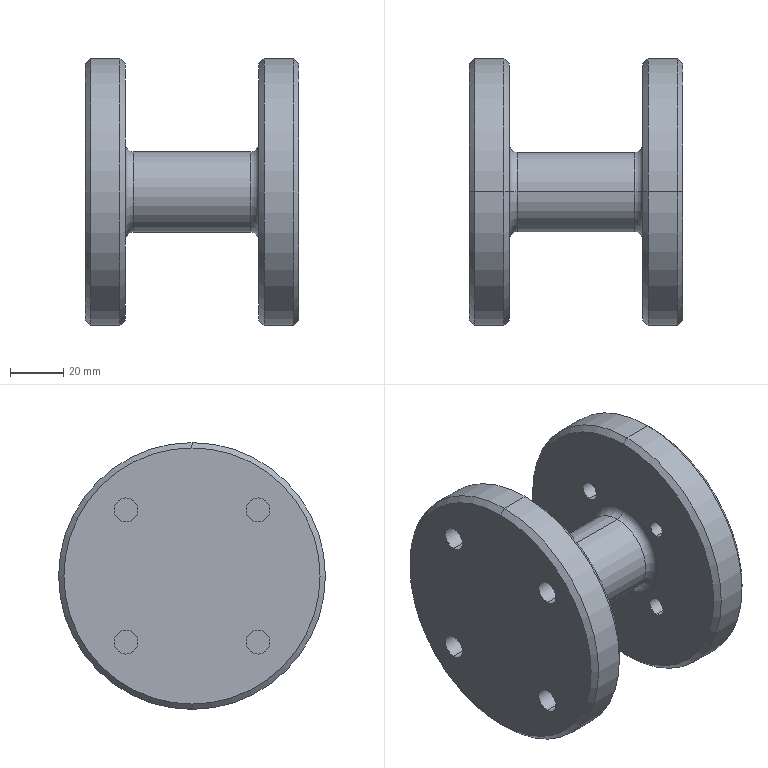Part | SolidWorks | features HoleWzd 3, ICE 2, Chamfer 1, CirPattern 1, Extrusion 1, Fillet 1 | 1 solid | 38 faces | box 80 x 100 x 100 mm | volume 263043 mm3 | cylinder 22 | cone 8 | torus 4 | plane 4 | commonest cylinder face diameters 9 x8 6 x4 7 x4 100 x4 30 x2
STEP:
#1=CARTESIAN_POINT('',(80.,0.,-48.));
#2=VERTEX_POINT('',#1);
#3=CARTESIAN_POINT('',(80.,0.,48.));
#4=VERTEX_POINT('',#3);
#5=CARTESIAN_POINT('',(80.,0.,0.));
#6=DIRECTION('',(1.,0.,0.));
#7=DIRECTION('',(0.,0.,-1.));
#8=AXIS2_PLACEMENT_3D('',#5,#6,#7);
#9=CIRCLE('',#8,48.);
#10=EDGE_CURVE('',#2,#4,#9,.T.);
#11=ORIENTED_EDGE('',*,*,#10,.F.);
#12=CARTESIAN_POINT('',(78.,0.,-50.));
#13=VERTEX_POINT('',#12);
#14=CARTESIAN_POINT('',(80.,0.,-48.));
#15=DIRECTION('',(-0.7071,0.,-0.7071));
#16=VECTOR('',#15,1000.);
#17=LINE('',#14,#16);
#18=EDGE_CURVE('',#2,#13,#17,.T.);
#19=ORIENTED_EDGE('',*,*,#18,.T.);
#20=CARTESIAN_POINT('',(78.,0.,50.));
#21=VERTEX_POINT('',#20);
#22=CARTESIAN_POINT('',(78.,0.,0.));
#23=DIRECTION('',(-1.,0.,0.));
#24=DIRECTION('',(0.,0.,-1.));
#25=AXIS2_PLACEMENT_3D('',#22,#23,#24);
#26=CIRCLE('',#25,50.);
#27=EDGE_CURVE('',#21,#13,#26,.T.);
#28=ORIENTED_EDGE('',*,*,#27,.F.);
#29=CARTESIAN_POINT('',(80.,0.,48.));
#30=DIRECTION('',(-0.7071,0.,0.7071));
#31=VECTOR('',#30,1000.);
#32=LINE('',#29,#31);
#33=EDGE_CURVE('',#4,#21,#32,.T.);
#34=ORIENTED_EDGE('',*,*,#33,.F.);
#35=EDGE_LOOP('',(#11,#19,#28,#34));
#36=FACE_OUTER_BOUND('',#35,.T.);
#37=CARTESIAN_POINT('',(80.,0.,0.));
#38=DIRECTION('',(-1.,0.,0.));
#39=DIRECTION('',(0.,0.,1.));
#40=AXIS2_PLACEMENT_3D('',#37,#38,#39);
#41=CONICAL_SURFACE('',#40,48.,0.7854);
#42=ADVANCED_FACE('',(#36),#41,.T.);
#43=CARTESIAN_POINT('',(65.,0.,48.));
#44=VERTEX_POINT('',#43);
#45=CARTESIAN_POINT('',(65.,0.,-48.));
#46=VERTEX_POINT('',#45);
#47=CARTESIAN_POINT('',(65.,0.,0.));
#48=DIRECTION('',(-1.,0.,0.));
#49=DIRECTION('',(0.,0.,-1.));
#50=AXIS2_PLACEMENT_3D('',#47,#48,#49);
#51=CIRCLE('',#50,48.);
#52=EDGE_CURVE('',#44,#46,#51,.T.);
#53=ORIENTED_EDGE('',*,*,#52,.F.);
#54=CARTESIAN_POINT('',(67.,0.,50.));
#55=VERTEX_POINT('',#54);
#56=CARTESIAN_POINT('',(67.,0.,50.));
#57=DIRECTION('',(0.7071,0.,0.7071));
#58=VECTOR('',#57,1000.);
#59=LINE('',#56,#58);
#60=EDGE_CURVE('',#44,#55,#59,.T.);
#61=ORIENTED_EDGE('',*,*,#60,.T.);
#62=CARTESIAN_POINT('',(67.,0.,-50.));
#63=VERTEX_POINT('',#62);
#64=CARTESIAN_POINT('',(67.,0.,0.));
#65=DIRECTION('',(1.,0.,0.));
#66=DIRECTION('',(0.,0.,-1.));
#67=AXIS2_PLACEMENT_3D('',#64,#65,#66);
#68=CIRCLE('',#67,50.);
#69=EDGE_CURVE('',#63,#55,#68,.T.);
#70=ORIENTED_EDGE('',*,*,#69,.F.);
#71=CARTESIAN_POINT('',(67.,0.,-50.));
#72=DIRECTION('',(0.7071,0.,-0.7071));
#73=VECTOR('',#72,1000.);
#74=LINE('',#71,#73);
#75=EDGE_CURVE('',#46,#63,#74,.T.);
#76=ORIENTED_EDGE('',*,*,#75,.F.);
#77=EDGE_LOOP('',(#53,#61,#70,#76));
#78=FACE_OUTER_BOUND('',#77,.T.);
#79=CARTESIAN_POINT('',(67.,0.,0.));
#80=DIRECTION('',(1.,0.,0.));
#81=DIRECTION('',(0.,0.,-1.));
#82=AXIS2_PLACEMENT_3D('',#79,#80,#81);
#83=CONICAL_SURFACE('',#82,50.,0.7854);
#84=ADVANCED_FACE('',(#78),#83,.T.);
#85=CARTESIAN_POINT('',(15.,0.,-48.));
#86=VERTEX_POINT('',#85);
#87=CARTESIAN_POINT('',(15.,0.,48.));
#88=VERTEX_POINT('',#87);
#89=CARTESIAN_POINT('',(15.,0.,0.));
#90=DIRECTION('',(1.,0.,0.));
#91=DIRECTION('',(0.,0.,-1.));
#92=AXIS2_PLACEMENT_3D('',#89,#90,#91);
#93=CIRCLE('',#92,48.);
#94=EDGE_CURVE('',#86,#88,#93,.T.);
#95=ORIENTED_EDGE('',*,*,#94,.F.);
#96=CARTESIAN_POINT('',(13.,0.,-50.));
#97=VERTEX_POINT('',#96);
#98=CARTESIAN_POINT('',(15.,0.,-48.));
#99=DIRECTION('',(-0.7071,0.,-0.7071));
#100=VECTOR('',#99,1000.);
#101=LINE('',#98,#100);
#102=EDGE_CURVE('',#86,#97,#101,.T.);
#103=ORIENTED_EDGE('',*,*,#102,.T.);
#104=CARTESIAN_POINT('',(13.,0.,50.));
#105=VERTEX_POINT('',#104);
#106=CARTESIAN_POINT('',(13.,0.,0.));
#107=DIRECTION('',(-1.,0.,0.));
#108=DIRECTION('',(0.,0.,-1.));
#109=AXIS2_PLACEMENT_3D('',#106,#107,#108);
#110=CIRCLE('',#109,50.);
#111=EDGE_CURVE('',#105,#97,#110,.T.);
#112=ORIENTED_EDGE('',*,*,#111,.F.);
#113=CARTESIAN_POINT('',(15.,0.,48.));
#114=DIRECTION('',(-0.7071,0.,0.7071));
#115=VECTOR('',#114,1000.);
#116=LINE('',#113,#115);
#117=EDGE_CURVE('',#88,#105,#116,.T.);
#118=ORIENTED_EDGE('',*,*,#117,.F.);
#119=EDGE_LOOP('',(#95,#103,#112,#118));
#120=FACE_OUTER_BOUND('',#119,.T.);
#121=CARTESIAN_POINT('',(15.,0.,0.));
#122=DIRECTION('',(-1.,0.,0.));
#123=DIRECTION('',(0.,0.,1.));
#124=AXIS2_PLACEMENT_3D('',#121,#122,#123);
#125=CONICAL_SURFACE('',#124,48.,0.7854);
#126=ADVANCED_FACE('',(#120),#125,.T.);
#127=CARTESIAN_POINT('',(0.,0.,48.));
#128=VERTEX_POINT('',#127);
#129=CARTESIAN_POINT('',(0.,0.,-48.));
#130=VERTEX_POINT('',#129);
#131=CARTESIAN_POINT('',(0.,0.,0.));
#132=DIRECTION('',(-1.,0.,0.));
#133=DIRECTION('',(0.,0.,-1.));
#134=AXIS2_PLACEMENT_3D('',#131,#132,#133);
#135=CIRCLE('',#134,48.);
#136=EDGE_CURVE('',#128,#130,#135,.T.);
#137=ORIENTED_EDGE('',*,*,#136,.F.);
#138=CARTESIAN_POINT('',(2.,0.,50.));
#139=VERTEX_POINT('',#138);
#140=CARTESIAN_POINT('',(2.,0.,50.));
#141=DIRECTION('',(0.7071,0.,0.7071));
#142=VECTOR('',#141,1000.);
#143=LINE('',#140,#142);
#144=EDGE_CURVE('',#128,#139,#143,.T.);
#145=ORIENTED_EDGE('',*,*,#144,.T.);
#146=CARTESIAN_POINT('',(2.,0.,-50.));
#147=VERTEX_POINT('',#146);
#148=CARTESIAN_POINT('',(2.,0.,0.));
#149=DIRECTION('',(1.,0.,0.));
#150=DIRECTION('',(0.,0.,-1.));
#151=AXIS2_PLACEMENT_3D('',#148,#149,#150);
#152=CIRCLE('',#151,50.);
#153=EDGE_CURVE('',#147,#139,#152,.T.);
#154=ORIENTED_EDGE('',*,*,#153,.F.);
#155=CARTESIAN_POINT('',(2.,0.,-50.));
#156=DIRECTION('',(0.7071,0.,-0.7071));
#157=VECTOR('',#156,1000.);
#158=LINE('',#155,#157);
#159=EDGE_CURVE('',#130,#147,#158,.T.);
#160=ORIENTED_EDGE('',*,*,#159,.F.);
#161=EDGE_LOOP('',(#137,#145,#154,#160));
#162=FACE_OUTER_BOUND('',#161,.T.);
#163=CARTESIAN_POINT('',(2.,0.,0.));
#164=DIRECTION('',(1.,0.,0.));
#165=DIRECTION('',(0.,0.,-1.));
#166=AXIS2_PLACEMENT_3D('',#163,#164,#165);
#167=CONICAL_SURFACE('',#166,50.,0.7854);
#168=ADVANCED_FACE('',(#162),#167,.T.);
#169=CARTESIAN_POINT('',(65.,0.,18.));
#170=VERTEX_POINT('',#169);
#171=CARTESIAN_POINT('',(65.,0.,-18.));
#172=VERTEX_POINT('',#171);
#173=CARTESIAN_POINT('',(65.,0.,0.));
#174=DIRECTION('',(1.,0.,0.));
#175=DIRECTION('',(0.,0.,-1.));
#176=AXIS2_PLACEMENT_3D('',#173,#174,#175);
#177=CIRCLE('',#176,18.);
#178=EDGE_CURVE('',#170,#172,#177,.T.);
#179=ORIENTED_EDGE('',*,*,#178,.F.);
#180=CARTESIAN_POINT('',(62.,0.,15.));
#181=VERTEX_POINT('',#180);
#182=CARTESIAN_POINT('',(62.,0.,18.));
#183=DIRECTION('',(0.,1.,0.));
#184=DIRECTION('',(0.,0.,1.));
#185=AXIS2_PLACEMENT_3D('',#182,#183,#184);
#186=CIRCLE('',#185,3.);
#187=EDGE_CURVE('',#170,#181,#186,.T.);
#188=ORIENTED_EDGE('',*,*,#187,.T.);
#189=CARTESIAN_POINT('',(62.,0.,-15.));
#190=VERTEX_POINT('',#189);
#191=CARTESIAN_POINT('',(62.,0.,0.));
#192=DIRECTION('',(-1.,0.,0.));
#193=DIRECTION('',(0.,0.,-1.));
#194=AXIS2_PLACEMENT_3D('',#191,#192,#193);
#195=CIRCLE('',#194,15.);
#196=EDGE_CURVE('',#190,#181,#195,.T.);
#197=ORIENTED_EDGE('',*,*,#196,.F.);
#198=CARTESIAN_POINT('',(62.,0.,-18.));
#199=DIRECTION('',(0.,-1.,0.));
#200=DIRECTION('',(0.,0.,-1.));
#201=AXIS2_PLACEMENT_3D('',#198,#199,#200);
#202=CIRCLE('',#201,3.);
#203=EDGE_CURVE('',#172,#190,#202,.T.);
#204=ORIENTED_EDGE('',*,*,#203,.F.);
#205=EDGE_LOOP('',(#179,#188,#197,#204));
#206=FACE_OUTER_BOUND('',#205,.T.);
#207=CARTESIAN_POINT('',(62.,0.,0.));
#208=DIRECTION('',(1.,0.,0.));
#209=DIRECTION('',(0.,0.,-1.));
#210=AXIS2_PLACEMENT_3D('',#207,#208,#209);
#211=TOROIDAL_SURFACE('',#210,18.,3.);
#212=ADVANCED_FACE('',(#206),#211,.F.);
#213=CARTESIAN_POINT('',(18.,0.,15.));
#214=VERTEX_POINT('',#213);
#215=CARTESIAN_POINT('',(18.,0.,-15.));
#216=VERTEX_POINT('',#215);
#217=CARTESIAN_POINT('',(18.,0.,0.));
#218=DIRECTION('',(1.,0.,0.));
#219=DIRECTION('',(0.,0.,-1.));
#220=AXIS2_PLACEMENT_3D('',#217,#218,#219);
#221=CIRCLE('',#220,15.);
#222=EDGE_CURVE('',#214,#216,#221,.T.);
#223=ORIENTED_EDGE('',*,*,#222,.F.);
#224=CARTESIAN_POINT('',(15.,0.,18.));
#225=VERTEX_POINT('',#224);
#226=CARTESIAN_POINT('',(18.,0.,18.));
#227=DIRECTION('',(0.,1.,0.));
#228=DIRECTION('',(0.,0.,1.));
#229=AXIS2_PLACEMENT_3D('',#226,#227,#228);
#230=CIRCLE('',#229,3.);
#231=EDGE_CURVE('',#214,#225,#230,.T.);
#232=ORIENTED_EDGE('',*,*,#231,.T.);
#233=CARTESIAN_POINT('',(15.,0.,-18.));
#234=VERTEX_POINT('',#233);
#235=CARTESIAN_POINT('',(15.,0.,0.));
#236=DIRECTION('',(-1.,0.,0.));
#237=DIRECTION('',(0.,0.,-1.));
#238=AXIS2_PLACEMENT_3D('',#235,#236,#237);
#239=CIRCLE('',#238,18.);
#240=EDGE_CURVE('',#234,#225,#239,.T.);
#241=ORIENTED_EDGE('',*,*,#240,.F.);
#242=CARTESIAN_POINT('',(18.,0.,-18.));
#243=DIRECTION('',(0.,-1.,0.));
#244=DIRECTION('',(0.,0.,-1.));
#245=AXIS2_PLACEMENT_3D('',#242,#243,#244);
#246=CIRCLE('',#245,3.);
#247=EDGE_CURVE('',#216,#234,#246,.T.);
#248=ORIENTED_EDGE('',*,*,#247,.F.);
#249=EDGE_LOOP('',(#223,#232,#241,#248));
#250=FACE_OUTER_BOUND('',#249,.T.);
#251=CARTESIAN_POINT('',(18.,0.,0.));
#252=DIRECTION('',(1.,0.,0.));
#253=DIRECTION('',(0.,0.,-1.));
#254=AXIS2_PLACEMENT_3D('',#251,#252,#253);
#255=TOROIDAL_SURFACE('',#254,18.,3.);
#256=ADVANCED_FACE('',(#250),#255,.F.);
#257=CARTESIAN_POINT('',(15.,24.749,29.249));
#258=VERTEX_POINT('',#257);
#259=CARTESIAN_POINT('',(15.,24.749,20.249));
#260=VERTEX_POINT('',#259);
#261=CARTESIAN_POINT('',(15.,24.749,24.749));
#262=DIRECTION('',(1.,0.,0.));
#263=DIRECTION('',(0.,0.,-1.));
#264=AXIS2_PLACEMENT_3D('',#261,#262,#263);
#265=CIRCLE('',#264,4.5);
#266=EDGE_CURVE('',#258,#260,#265,.T.);
#267=ORIENTED_EDGE('',*,*,#266,.T.);
#268=CARTESIAN_POINT('',(0.,24.749,20.249));
#269=VERTEX_POINT('',#268);
#270=CARTESIAN_POINT('',(0.,24.749,20.249));
#271=DIRECTION('',(-1.,0.,0.));
#272=VECTOR('',#271,1000.);
#273=LINE('',#270,#272);
#274=EDGE_CURVE('',#260,#269,#273,.T.);
#275=ORIENTED_EDGE('',*,*,#274,.T.);
#276=CARTESIAN_POINT('',(0.,24.749,29.249));
#277=VERTEX_POINT('',#276);
#278=CARTESIAN_POINT('',(0.,24.749,24.749));
#279=DIRECTION('',(-1.,0.,0.));
#280=DIRECTION('',(0.,0.,1.));
#281=AXIS2_PLACEMENT_3D('',#278,#279,#280);
#282=CIRCLE('',#281,4.5);
#283=EDGE_CURVE('',#269,#277,#282,.T.);
#284=ORIENTED_EDGE('',*,*,#283,.T.);
#285=CARTESIAN_POINT('',(0.,24.749,29.249));
#286=DIRECTION('',(-1.,0.,0.));
#287=VECTOR('',#286,1000.);
#288=LINE('',#285,#287);
#289=EDGE_CURVE('',#258,#277,#288,.T.);
#290=ORIENTED_EDGE('',*,*,#289,.F.);
#291=EDGE_LOOP('',(#267,#275,#284,#290));
#292=FACE_OUTER_BOUND('',#291,.T.);
#293=CARTESIAN_POINT('',(0.,24.749,24.749));
#294=DIRECTION('',(-1.,0.,0.));
#295=DIRECTION('',(0.,0.,1.));
#296=AXIS2_PLACEMENT_3D('',#293,#294,#295);
#297=CYLINDRICAL_SURFACE('',#296,4.5);
#298=ADVANCED_FACE('',(#292),#297,.F.);
#299=CARTESIAN_POINT('',(15.,-24.749,29.249));
#300=VERTEX_POINT('',#299);
#301=CARTESIAN_POINT('',(15.,-24.749,20.249));
#302=VERTEX_POINT('',#301);
#303=CARTESIAN_POINT('',(15.,-24.749,24.749));
#304=DIRECTION('',(1.,0.,0.));
#305=DIRECTION('',(0.,0.,-1.));
#306=AXIS2_PLACEMENT_3D('',#303,#304,#305);
#307=CIRCLE('',#306,4.5);
#308=EDGE_CURVE('',#300,#302,#307,.T.);
#309=ORIENTED_EDGE('',*,*,#308,.T.);
#310=CARTESIAN_POINT('',(0.,-24.749,20.249));
#311=VERTEX_POINT('',#310);
#312=CARTESIAN_POINT('',(0.,-24.749,20.249));
#313=DIRECTION('',(-1.,0.,0.));
#314=VECTOR('',#313,1000.);
#315=LINE('',#312,#314);
#316=EDGE_CURVE('',#302,#311,#315,.T.);
#317=ORIENTED_EDGE('',*,*,#316,.T.);
#318=CARTESIAN_POINT('',(0.,-24.749,29.249));
#319=VERTEX_POINT('',#318);
#320=CARTESIAN_POINT('',(0.,-24.749,24.749));
#321=DIRECTION('',(-1.,0.,0.));
#322=DIRECTION('',(0.,0.,1.));
#323=AXIS2_PLACEMENT_3D('',#320,#321,#322);
#324=CIRCLE('',#323,4.5);
#325=EDGE_CURVE('',#311,#319,#324,.T.);
#326=ORIENTED_EDGE('',*,*,#325,.T.);
#327=CARTESIAN_POINT('',(0.,-24.749,29.249));
#328=DIRECTION('',(-1.,0.,0.));
#329=VECTOR('',#328,1000.);
#330=LINE('',#327,#329);
#331=EDGE_CURVE('',#300,#319,#330,.T.);
#332=ORIENTED_EDGE('',*,*,#331,.F.);
#333=EDGE_LOOP('',(#309,#317,#326,#332));
#334=FACE_OUTER_BOUND('',#333,.T.);
#335=CARTESIAN_POINT('',(0.,-24.749,24.749));
#336=DIRECTION('',(-1.,0.,0.));
#337=DIRECTION('',(0.,0.,1.));
#338=AXIS2_PLACEMENT_3D('',#335,#336,#337);
#339=CYLINDRICAL_SURFACE('',#338,4.5);
#340=ADVANCED_FACE('',(#334),#339,.F.);
#341=CARTESIAN_POINT('',(15.,-24.749,-20.249));
#342=VERTEX_POINT('',#341);
#343=CARTESIAN_POINT('',(15.,-24.749,-29.249));
#344=VERTEX_POINT('',#343);
#345=CARTESIAN_POINT('',(15.,-24.749,-24.749));
#346=DIRECTION('',(1.,0.,0.));
#347=DIRECTION('',(0.,0.,-1.));
#348=AXIS2_PLACEMENT_3D('',#345,#346,#347);
#349=CIRCLE('',#348,4.5);
#350=EDGE_CURVE('',#342,#344,#349,.T.);
#351=ORIENTED_EDGE('',*,*,#350,.T.);
#352=CARTESIAN_POINT('',(0.,-24.749,-29.249));
#353=VERTEX_POINT('',#352);
#354=CARTESIAN_POINT('',(0.,-24.749,-29.249));
#355=DIRECTION('',(-1.,0.,0.));
#356=VECTOR('',#355,1000.);
#357=LINE('',#354,#356);
#358=EDGE_CURVE('',#344,#353,#357,.T.);
#359=ORIENTED_EDGE('',*,*,#358,.T.);
#360=CARTESIAN_POINT('',(0.,-24.749,-20.249));
#361=VERTEX_POINT('',#360);
#362=CARTESIAN_POINT('',(0.,-24.749,-24.749));
#363=DIRECTION('',(-1.,0.,0.));
#364=DIRECTION('',(0.,0.,1.));
#365=AXIS2_PLACEMENT_3D('',#362,#363,#364);
#366=CIRCLE('',#365,4.5);
#367=EDGE_CURVE('',#353,#361,#366,.T.);
#368=ORIENTED_EDGE('',*,*,#367,.T.);
#369=CARTESIAN_POINT('',(0.,-24.749,-20.249));
#370=DIRECTION('',(-1.,0.,0.));
#371=VECTOR('',#370,1000.);
#372=LINE('',#369,#371);
#373=EDGE_CURVE('',#342,#361,#372,.T.);
#374=ORIENTED_EDGE('',*,*,#373,.F.);
#375=EDGE_LOOP('',(#351,#359,#368,#374));
#376=FACE_OUTER_BOUND('',#375,.T.);
#377=CARTESIAN_POINT('',(0.,-24.749,-24.749));
#378=DIRECTION('',(-1.,0.,0.));
#379=DIRECTION('',(0.,0.,1.));
#380=AXIS2_PLACEMENT_3D('',#377,#378,#379);
#381=CYLINDRICAL_SURFACE('',#380,4.5);
#382=ADVANCED_FACE('',(#376),#381,.F.);
#383=CARTESIAN_POINT('',(15.,24.749,-20.249));
#384=VERTEX_POINT('',#383);
#385=CARTESIAN_POINT('',(15.,24.749,-29.249));
#386=VERTEX_POINT('',#385);
#387=CARTESIAN_POINT('',(15.,24.749,-24.749));
#388=DIRECTION('',(1.,0.,0.));
#389=DIRECTION('',(0.,0.,-1.));
#390=AXIS2_PLACEMENT_3D('',#387,#388,#389);
#391=CIRCLE('',#390,4.5);
#392=EDGE_CURVE('',#384,#386,#391,.T.);
#393=ORIENTED_EDGE('',*,*,#392,.T.);
#394=CARTESIAN_POINT('',(0.,24.749,-29.249));
#395=VERTEX_POINT('',#394);
#396=CARTESIAN_POINT('',(0.,24.749,-29.249));
#397=DIRECTION('',(-1.,0.,0.));
#398=VECTOR('',#397,1000.);
#399=LINE('',#396,#398);
#400=EDGE_CURVE('',#386,#395,#399,.T.);
#401=ORIENTED_EDGE('',*,*,#400,.T.);
#402=CARTESIAN_POINT('',(0.,24.749,-20.249));
#403=VERTEX_POINT('',#402);
#404=CARTESIAN_POINT('',(0.,24.749,-24.749));
#405=DIRECTION('',(-1.,0.,0.));
#406=DIRECTION('',(0.,0.,1.));
#407=AXIS2_PLACEMENT_3D('',#404,#405,#406);
#408=CIRCLE('',#407,4.5);
#409=EDGE_CURVE('',#395,#403,#408,.T.);
#410=ORIENTED_EDGE('',*,*,#409,.T.);
#411=CARTESIAN_POINT('',(0.,24.749,-20.249));
#412=DIRECTION('',(-1.,0.,0.));
#413=VECTOR('',#412,1000.);
#414=LINE('',#411,#413);
#415=EDGE_CURVE('',#384,#403,#414,.T.);
#416=ORIENTED_EDGE('',*,*,#415,.F.);
#417=EDGE_LOOP('',(#393,#401,#410,#416));
#418=FACE_OUTER_BOUND('',#417,.T.);
#419=CARTESIAN_POINT('',(0.,24.749,-24.749));
#420=DIRECTION('',(-1.,0.,0.));
#421=DIRECTION('',(0.,0.,1.));
#422=AXIS2_PLACEMENT_3D('',#419,#420,#421);
#423=CYLINDRICAL_SURFACE('',#422,4.5);
#424=ADVANCED_FACE('',(#418),#423,.F.);
#425=CARTESIAN_POINT('',(65.,-17.699,20.699));
#426=VERTEX_POINT('',#425);
#427=CARTESIAN_POINT('',(65.,-17.699,14.699));
#428=VERTEX_POINT('',#427);
#429=CARTESIAN_POINT('',(65.,-17.699,17.699));
#430=DIRECTION('',(1.,0.,0.));
#431=DIRECTION('',(0.,0.,-1.));
#432=AXIS2_PLACEMENT_3D('',#429,#430,#431);
#433=CIRCLE('',#432,3.);
#434=EDGE_CURVE('',#426,#428,#433,.T.);
#435=ORIENTED_EDGE('',*,*,#434,.F.);
#436=CARTESIAN_POINT('',(80.,-17.699,20.699));
#437=VERTEX_POINT('',#436);
#438=CARTESIAN_POINT('',(80.,-17.699,20.699));
#439=DIRECTION('',(1.,0.,0.));
#440=VECTOR('',#439,1000.);
#441=LINE('',#438,#440);
#442=EDGE_CURVE('',#426,#437,#441,.T.);
#443=ORIENTED_EDGE('',*,*,#442,.T.);
#444=CARTESIAN_POINT('',(80.,-17.699,14.699));
#445=VERTEX_POINT('',#444);
#446=CARTESIAN_POINT('',(80.,-17.699,17.699));
#447=DIRECTION('',(1.,0.,0.));
#448=DIRECTION('',(0.,0.,-1.));
#449=AXIS2_PLACEMENT_3D('',#446,#447,#448);
#450=CIRCLE('',#449,3.);
#451=EDGE_CURVE('',#437,#445,#450,.T.);
#452=ORIENTED_EDGE('',*,*,#451,.T.);
#453=CARTESIAN_POINT('',(80.,-17.699,14.699));
#454=DIRECTION('',(1.,0.,0.));
#455=VECTOR('',#454,1000.);
#456=LINE('',#453,#455);
#457=EDGE_CURVE('',#428,#445,#456,.T.);
#458=ORIENTED_EDGE('',*,*,#457,.F.);
#459=EDGE_LOOP('',(#435,#443,#452,#458));
#460=FACE_OUTER_BOUND('',#459,.T.);
#461=CARTESIAN_POINT('',(80.,-17.699,17.699));
#462=DIRECTION('',(1.,0.,0.));
#463=DIRECTION('',(0.,0.,-1.));
#464=AXIS2_PLACEMENT_3D('',#461,#462,#463);
#465=CYLINDRICAL_SURFACE('',#464,3.);
#466=ADVANCED_FACE('',(#460),#465,.F.);
#467=CARTESIAN_POINT('',(65.,17.699,-14.699));
#468=VERTEX_POINT('',#467);
#469=CARTESIAN_POINT('',(65.,17.699,-20.699));
#470=VERTEX_POINT('',#469);
#471=CARTESIAN_POINT('',(65.,17.699,-17.699));
#472=DIRECTION('',(1.,0.,0.));
#473=DIRECTION('',(0.,0.,-1.));
#474=AXIS2_PLACEMENT_3D('',#471,#472,#473);
#475=CIRCLE('',#474,3.);
#476=EDGE_CURVE('',#468,#470,#475,.T.);
#477=ORIENTED_EDGE('',*,*,#476,.F.);
#478=CARTESIAN_POINT('',(80.,17.699,-14.699));
#479=VERTEX_POINT('',#478);
#480=CARTESIAN_POINT('',(80.,17.699,-14.699));
#481=DIRECTION('',(1.,0.,0.));
#482=VECTOR('',#481,1000.);
#483=LINE('',#480,#482);
#484=EDGE_CURVE('',#468,#479,#483,.T.);
#485=ORIENTED_EDGE('',*,*,#484,.T.);
#486=CARTESIAN_POINT('',(80.,17.699,-20.699));
#487=VERTEX_POINT('',#486);
#488=CARTESIAN_POINT('',(80.,17.699,-17.699));
#489=DIRECTION('',(1.,0.,0.));
#490=DIRECTION('',(0.,0.,-1.));
#491=AXIS2_PLACEMENT_3D('',#488,#489,#490);
#492=CIRCLE('',#491,3.);
#493=EDGE_CURVE('',#479,#487,#492,.T.);
#494=ORIENTED_EDGE('',*,*,#493,.T.);
#495=CARTESIAN_POINT('',(80.,17.699,-20.699));
#496=DIRECTION('',(1.,0.,0.));
#497=VECTOR('',#496,1000.);
#498=LINE('',#495,#497);
#499=EDGE_CURVE('',#470,#487,#498,.T.);
#500=ORIENTED_EDGE('',*,*,#499,.F.);
#501=EDGE_LOOP('',(#477,#485,#494,#500));
#502=FACE_OUTER_BOUND('',#501,.T.);
#503=CARTESIAN_POINT('',(80.,17.699,-17.699));
#504=DIRECTION('',(1.,0.,0.));
#505=DIRECTION('',(0.,0.,-1.));
#506=AXIS2_PLACEMENT_3D('',#503,#504,#505);
#507=CYLINDRICAL_SURFACE('',#506,3.);
#508=ADVANCED_FACE('',(#502),#507,.F.);
#509=CARTESIAN_POINT('',(65.,17.699,21.199));
#510=VERTEX_POINT('',#509);
#511=CARTESIAN_POINT('',(65.,17.699,14.199));
#512=VERTEX_POINT('',#511);
#513=CARTESIAN_POINT('',(65.,17.699,17.699));
#514=DIRECTION('',(1.,0.,0.));
#515=DIRECTION('',(0.,0.,-1.));
#516=AXIS2_PLACEMENT_3D('',#513,#514,#515);
#517=CIRCLE('',#516,3.5);
#518=EDGE_CURVE('',#510,#512,#517,.T.);
#519=ORIENTED_EDGE('',*,*,#518,.F.);
#520=CARTESIAN_POINT('',(80.,17.699,21.199));
#521=VERTEX_POINT('',#520);
#522=CARTESIAN_POINT('',(80.,17.699,21.199));
#523=DIRECTION('',(1.,0.,0.));
#524=VECTOR('',#523,1000.);
#525=LINE('',#522,#524);
#526=EDGE_CURVE('',#510,#521,#525,.T.);
#527=ORIENTED_EDGE('',*,*,#526,.T.);
#528=CARTESIAN_POINT('',(80.,17.699,14.199));
#529=VERTEX_POINT('',#528);
#530=CARTESIAN_POINT('',(80.,17.699,17.699));
#531=DIRECTION('',(1.,0.,0.));
#532=DIRECTION('',(0.,0.,-1.));
#533=AXIS2_PLACEMENT_3D('',#530,#531,#532);
#534=CIRCLE('',#533,3.5);
#535=EDGE_CURVE('',#521,#529,#534,.T.);
#536=ORIENTED_EDGE('',*,*,#535,.T.);
#537=CARTESIAN_POINT('',(80.,17.699,14.199));
#538=DIRECTION('',(1.,0.,0.));
#539=VECTOR('',#538,1000.);
#540=LINE('',#537,#539);
#541=EDGE_CURVE('',#512,#529,#540,.T.);
#542=ORIENTED_EDGE('',*,*,#541,.F.);
#543=EDGE_LOOP('',(#519,#527,#536,#542));
#544=FACE_OUTER_BOUND('',#543,.T.);
#545=CARTESIAN_POINT('',(80.,17.699,17.699));
#546=DIRECTION('',(1.,0.,0.));
#547=DIRECTION('',(0.,0.,-1.));
#548=AXIS2_PLACEMENT_3D('',#545,#546,#547);
#549=CYLINDRICAL_SURFACE('',#548,3.5);
#550=ADVANCED_FACE('',(#544),#549,.F.);
#551=CARTESIAN_POINT('',(65.,-17.699,-14.199));
#552=VERTEX_POINT('',#551);
#553=CARTESIAN_POINT('',(65.,-17.699,-21.199));
#554=VERTEX_POINT('',#553);
#555=CARTESIAN_POINT('',(65.,-17.699,-17.699));
#556=DIRECTION('',(1.,0.,0.));
#557=DIRECTION('',(0.,0.,-1.));
#558=AXIS2_PLACEMENT_3D('',#555,#556,#557);
#559=CIRCLE('',#558,3.5);
#560=EDGE_CURVE('',#552,#554,#559,.T.);
#561=ORIENTED_EDGE('',*,*,#560,.F.);
#562=CARTESIAN_POINT('',(80.,-17.699,-14.199));
#563=VERTEX_POINT('',#562);
#564=CARTESIAN_POINT('',(80.,-17.699,-14.199));
#565=DIRECTION('',(1.,0.,0.));
#566=VECTOR('',#565,1000.);
#567=LINE('',#564,#566);
#568=EDGE_CURVE('',#552,#563,#567,.T.);
#569=ORIENTED_EDGE('',*,*,#568,.T.);
#570=CARTESIAN_POINT('',(80.,-17.699,-21.199));
#571=VERTEX_POINT('',#570);
#572=CARTESIAN_POINT('',(80.,-17.699,-17.699));
#573=DIRECTION('',(1.,0.,0.));
#574=DIRECTION('',(0.,0.,-1.));
#575=AXIS2_PLACEMENT_3D('',#572,#573,#574);
#576=CIRCLE('',#575,3.5);
#577=EDGE_CURVE('',#563,#571,#576,.T.);
#578=ORIENTED_EDGE('',*,*,#577,.T.);
#579=CARTESIAN_POINT('',(80.,-17.699,-21.199));
#580=DIRECTION('',(1.,0.,0.));
#581=VECTOR('',#580,1000.);
#582=LINE('',#579,#581);
#583=EDGE_CURVE('',#554,#571,#582,.T.);
#584=ORIENTED_EDGE('',*,*,#583,.F.);
#585=EDGE_LOOP('',(#561,#569,#578,#584));
#586=FACE_OUTER_BOUND('',#585,.T.);
#587=CARTESIAN_POINT('',(80.,-17.699,-17.699));
#588=DIRECTION('',(1.,0.,0.));
#589=DIRECTION('',(0.,0.,-1.));
#590=AXIS2_PLACEMENT_3D('',#587,#588,#589);
#591=CYLINDRICAL_SURFACE('',#590,3.5);
#592=ADVANCED_FACE('',(#586),#591,.F.);
#593=ORIENTED_EDGE('',*,*,#27,.T.);
#594=CARTESIAN_POINT('',(80.,0.,-50.));
#595=DIRECTION('',(-1.,0.,0.));
#596=VECTOR('',#595,1000.);
#597=LINE('',#594,#596);
#598=EDGE_CURVE('',#13,#63,#597,.T.);
#599=ORIENTED_EDGE('',*,*,#598,.T.);
#600=ORIENTED_EDGE('',*,*,#69,.T.);
#601=CARTESIAN_POINT('',(80.,0.,50.));
#602=DIRECTION('',(-1.,0.,0.));
#603=VECTOR('',#602,1000.);
#604=LINE('',#601,#603);
#605=EDGE_CURVE('',#21,#55,#604,.T.);
#606=ORIENTED_EDGE('',*,*,#605,.F.);
#607=EDGE_LOOP('',(#593,#599,#600,#606));
#608=FACE_OUTER_BOUND('',#607,.T.);
#609=CARTESIAN_POINT('',(80.,0.,0.));
#610=DIRECTION('',(-1.,0.,0.));
#611=DIRECTION('',(0.,0.,1.));
#612=AXIS2_PLACEMENT_3D('',#609,#610,#611);
#613=CYLINDRICAL_SURFACE('',#612,50.);
#614=ADVANCED_FACE('',(#608),#613,.T.);
#615=CARTESIAN_POINT('',(62.,0.,0.));
#616=DIRECTION('',(-1.,0.,0.));
#617=DIRECTION('',(0.,0.,-1.));
#618=AXIS2_PLACEMENT_3D('',#615,#616,#617);
#619=CIRCLE('',#618,15.);
#620=EDGE_CURVE('',#181,#190,#619,.T.);
#621=ORIENTED_EDGE('',*,*,#620,.T.);
#622=CARTESIAN_POINT('',(65.,0.,-15.));
#623=DIRECTION('',(-1.,0.,0.));
#624=VECTOR('',#623,1000.);
#625=LINE('',#622,#624);
#626=EDGE_CURVE('',#190,#216,#625,.T.);
#627=ORIENTED_EDGE('',*,*,#626,.T.);
#628=CARTESIAN_POINT('',(18.,0.,0.));
#629=DIRECTION('',(1.,0.,0.));
#630=DIRECTION('',(0.,0.,-1.));
#631=AXIS2_PLACEMENT_3D('',#628,#629,#630);
#632=CIRCLE('',#631,15.);
#633=EDGE_CURVE('',#216,#214,#632,.T.);
#634=ORIENTED_EDGE('',*,*,#633,.T.);
#635=CARTESIAN_POINT('',(65.,0.,15.));
#636=DIRECTION('',(-1.,0.,0.));
#637=VECTOR('',#636,1000.);
#638=LINE('',#635,#637);
#639=EDGE_CURVE('',#181,#214,#638,.T.);
#640=ORIENTED_EDGE('',*,*,#639,.F.);
#641=EDGE_LOOP('',(#621,#627,#634,#640));
#642=FACE_OUTER_BOUND('',#641,.T.);
#643=CARTESIAN_POINT('',(65.,0.,0.));
#644=DIRECTION('',(-1.,0.,0.));
#645=DIRECTION('',(0.,0.,1.));
#646=AXIS2_PLACEMENT_3D('',#643,#644,#645);
#647=CYLINDRICAL_SURFACE('',#646,15.);
#648=ADVANCED_FACE('',(#642),#647,.T.);
#649=ORIENTED_EDGE('',*,*,#111,.T.);
#650=CARTESIAN_POINT('',(15.,0.,-50.));
#651=DIRECTION('',(-1.,0.,0.));
#652=VECTOR('',#651,1000.);
#653=LINE('',#650,#652);
#654=EDGE_CURVE('',#97,#147,#653,.T.);
#655=ORIENTED_EDGE('',*,*,#654,.T.);
#656=ORIENTED_EDGE('',*,*,#153,.T.);
#657=CARTESIAN_POINT('',(15.,0.,50.));
#658=DIRECTION('',(-1.,0.,0.));
#659=VECTOR('',#658,1000.);
#660=LINE('',#657,#659);
#661=EDGE_CURVE('',#105,#139,#660,.T.);
#662=ORIENTED_EDGE('',*,*,#661,.F.);
#663=EDGE_LOOP('',(#649,#655,#656,#662));
#664=FACE_OUTER_BOUND('',#663,.T.);
#665=CARTESIAN_POINT('',(15.,0.,0.));
#666=DIRECTION('',(-1.,0.,0.));
#667=DIRECTION('',(0.,0.,1.));
#668=AXIS2_PLACEMENT_3D('',#665,#666,#667);
#669=CYLINDRICAL_SURFACE('',#668,50.);
#670=ADVANCED_FACE('',(#664),#669,.T.);
#671=ORIENTED_EDGE('',*,*,#654,.F.);
#672=CARTESIAN_POINT('',(13.,0.,0.));
#673=DIRECTION('',(-1.,0.,0.));
#674=DIRECTION('',(0.,0.,-1.));
#675=AXIS2_PLACEMENT_3D('',#672,#673,#674);
#676=CIRCLE('',#675,50.);
#677=EDGE_CURVE('',#97,#105,#676,.T.);
#678=ORIENTED_EDGE('',*,*,#677,.T.);
#679=ORIENTED_EDGE('',*,*,#661,.T.);
#680=CARTESIAN_POINT('',(2.,0.,0.));
#681=DIRECTION('',(1.,0.,0.));
#682=DIRECTION('',(0.,0.,-1.));
#683=AXIS2_PLACEMENT_3D('',#680,#681,#682);
#684=CIRCLE('',#683,50.);
#685=EDGE_CURVE('',#139,#147,#684,.T.);
#686=ORIENTED_EDGE('',*,*,#685,.T.);
#687=EDGE_LOOP('',(#671,#678,#679,#686));
#688=FACE_OUTER_BOUND('',#687,.T.);
#689=CARTESIAN_POINT('',(15.,0.,0.));
#690=DIRECTION('',(-1.,0.,0.));
#691=DIRECTION('',(0.,0.,1.));
#692=AXIS2_PLACEMENT_3D('',#689,#690,#691);
#693=CYLINDRICAL_SURFACE('',#692,50.);
#694=ADVANCED_FACE('',(#688),#693,.T.);
#695=CARTESIAN_POINT('',(15.,0.,0.));
#696=DIRECTION('',(1.,0.,0.));
#697=DIRECTION('',(0.,0.,-1.));
#698=AXIS2_PLACEMENT_3D('',#695,#696,#697);
#699=CIRCLE('',#698,48.);
#700=EDGE_CURVE('',#88,#86,#699,.T.);
#701=ORIENTED_EDGE('',*,*,#700,.T.);
#702=ORIENTED_EDGE('',*,*,#94,.T.);
#703=EDGE_LOOP('',(#701,#702));
#704=FACE_OUTER_BOUND('',#703,.T.);
#705=ORIENTED_EDGE('',*,*,#240,.T.);
#706=CARTESIAN_POINT('',(15.,0.,0.));
#707=DIRECTION('',(-1.,0.,0.));
#708=DIRECTION('',(0.,0.,-1.));
#709=AXIS2_PLACEMENT_3D('',#706,#707,#708);
#710=CIRCLE('',#709,18.);
#711=EDGE_CURVE('',#225,#234,#710,.T.);
#712=ORIENTED_EDGE('',*,*,#711,.T.);
#713=EDGE_LOOP('',(#705,#712));
#714=FACE_BOUND('',#713,.T.);
#715=ORIENTED_EDGE('',*,*,#266,.F.);
#716=CARTESIAN_POINT('',(15.,24.749,24.749));
#717=DIRECTION('',(1.,0.,0.));
#718=DIRECTION('',(0.,0.,-1.));
#719=AXIS2_PLACEMENT_3D('',#716,#717,#718);
#720=CIRCLE('',#719,4.5);
#721=EDGE_CURVE('',#260,#258,#720,.T.);
#722=ORIENTED_EDGE('',*,*,#721,.F.);
#723=EDGE_LOOP('',(#715,#722));
#724=FACE_BOUND('',#723,.T.);
#725=ORIENTED_EDGE('',*,*,#308,.F.);
#726=CARTESIAN_POINT('',(15.,-24.749,24.749));
#727=DIRECTION('',(1.,0.,0.));
#728=DIRECTION('',(0.,0.,-1.));
#729=AXIS2_PLACEMENT_3D('',#726,#727,#728);
#730=CIRCLE('',#729,4.5);
#731=EDGE_CURVE('',#302,#300,#730,.T.);
#732=ORIENTED_EDGE('',*,*,#731,.F.);
#733=EDGE_LOOP('',(#725,#732));
#734=FACE_BOUND('',#733,.T.);
#735=ORIENTED_EDGE('',*,*,#350,.F.);
#736=CARTESIAN_POINT('',(15.,-24.749,-24.749));
#737=DIRECTION('',(1.,0.,0.));
#738=DIRECTION('',(0.,0.,-1.));
#739=AXIS2_PLACEMENT_3D('',#736,#737,#738);
#740=CIRCLE('',#739,4.5);
#741=EDGE_CURVE('',#344,#342,#740,.T.);
#742=ORIENTED_EDGE('',*,*,#741,.F.);
#743=EDGE_LOOP('',(#735,#742));
#744=FACE_BOUND('',#743,.T.);
#745=ORIENTED_EDGE('',*,*,#392,.F.);
#746=CARTESIAN_POINT('',(15.,24.749,-24.749));
#747=DIRECTION('',(1.,0.,0.));
#748=DIRECTION('',(0.,0.,-1.));
#749=AXIS2_PLACEMENT_3D('',#746,#747,#748);
#750=CIRCLE('',#749,4.5);
#751=EDGE_CURVE('',#386,#384,#750,.T.);
#752=ORIENTED_EDGE('',*,*,#751,.F.);
#753=EDGE_LOOP('',(#745,#752));
#754=FACE_BOUND('',#753,.T.);
#755=CARTESIAN_POINT('',(15.,0.,0.));
#756=DIRECTION('',(1.,0.,0.));
#757=DIRECTION('',(0.,0.,-1.));
#758=AXIS2_PLACEMENT_3D('',#755,#756,#757);
#759=PLANE('',#758);
#760=ADVANCED_FACE('',(#704,#714,#724,#734,#744,#754),#759,.T.);
#761=CARTESIAN_POINT('',(0.,0.,0.));
#762=DIRECTION('',(-1.,0.,0.));
#763=DIRECTION('',(0.,0.,-1.));
#764=AXIS2_PLACEMENT_3D('',#761,#762,#763);
#765=CIRCLE('',#764,48.);
#766=EDGE_CURVE('',#130,#128,#765,.T.);
#767=ORIENTED_EDGE('',*,*,#766,.T.);
#768=ORIENTED_EDGE('',*,*,#136,.T.);
#769=EDGE_LOOP('',(#767,#768));
#770=FACE_OUTER_BOUND('',#769,.T.);
#771=CARTESIAN_POINT('',(0.,24.749,24.749));
#772=DIRECTION('',(-1.,0.,0.));
#773=DIRECTION('',(0.,0.,1.));
#774=AXIS2_PLACEMENT_3D('',#771,#772,#773);
#775=CIRCLE('',#774,4.5);
#776=EDGE_CURVE('',#277,#269,#775,.T.);
#777=ORIENTED_EDGE('',*,*,#776,.F.);
#778=ORIENTED_EDGE('',*,*,#283,.F.);
#779=EDGE_LOOP('',(#777,#778));
#780=FACE_BOUND('',#779,.T.);
#781=CARTESIAN_POINT('',(0.,-24.749,24.749));
#782=DIRECTION('',(-1.,0.,0.));
#783=DIRECTION('',(0.,0.,1.));
#784=AXIS2_PLACEMENT_3D('',#781,#782,#783);
#785=CIRCLE('',#784,4.5);
#786=EDGE_CURVE('',#319,#311,#785,.T.);
#787=ORIENTED_EDGE('',*,*,#786,.F.);
#788=ORIENTED_EDGE('',*,*,#325,.F.);
#789=EDGE_LOOP('',(#787,#788));
#790=FACE_BOUND('',#789,.T.);
#791=CARTESIAN_POINT('',(0.,-24.749,-24.749));
#792=DIRECTION('',(-1.,0.,0.));
#793=DIRECTION('',(0.,0.,1.));
#794=AXIS2_PLACEMENT_3D('',#791,#792,#793);
#795=CIRCLE('',#794,4.5);
#796=EDGE_CURVE('',#361,#353,#795,.T.);
#797=ORIENTED_EDGE('',*,*,#796,.F.);
#798=ORIENTED_EDGE('',*,*,#367,.F.);
#799=EDGE_LOOP('',(#797,#798));
#800=FACE_BOUND('',#799,.T.);
#801=CARTESIAN_POINT('',(0.,24.749,-24.749));
#802=DIRECTION('',(-1.,0.,0.));
#803=DIRECTION('',(0.,0.,1.));
#804=AXIS2_PLACEMENT_3D('',#801,#802,#803);
#805=CIRCLE('',#804,4.5);
#806=EDGE_CURVE('',#403,#395,#805,.T.);
#807=ORIENTED_EDGE('',*,*,#806,.F.);
#808=ORIENTED_EDGE('',*,*,#409,.F.);
#809=EDGE_LOOP('',(#807,#808));
#810=FACE_BOUND('',#809,.T.);
#811=CARTESIAN_POINT('',(0.,0.,0.));
#812=DIRECTION('',(1.,0.,0.));
#813=DIRECTION('',(0.,0.,-1.));
#814=AXIS2_PLACEMENT_3D('',#811,#812,#813);
#815=PLANE('',#814);
#816=ADVANCED_FACE('',(#770,#780,#790,#800,#810),#815,.F.);
#817=ORIENTED_EDGE('',*,*,#626,.F.);
#818=ORIENTED_EDGE('',*,*,#196,.T.);
#819=ORIENTED_EDGE('',*,*,#639,.T.);
#820=ORIENTED_EDGE('',*,*,#222,.T.);
#821=EDGE_LOOP('',(#817,#818,#819,#820));
#822=FACE_OUTER_BOUND('',#821,.T.);
#823=CARTESIAN_POINT('',(65.,0.,0.));
#824=DIRECTION('',(-1.,0.,0.));
#825=DIRECTION('',(0.,0.,1.));
#826=AXIS2_PLACEMENT_3D('',#823,#824,#825);
#827=CYLINDRICAL_SURFACE('',#826,15.);
#828=ADVANCED_FACE('',(#822),#827,.T.);
#829=ORIENTED_EDGE('',*,*,#598,.F.);
#830=CARTESIAN_POINT('',(78.,0.,0.));
#831=DIRECTION('',(-1.,0.,0.));
#832=DIRECTION('',(0.,0.,-1.));
#833=AXIS2_PLACEMENT_3D('',#830,#831,#832);
#834=CIRCLE('',#833,50.);
#835=EDGE_CURVE('',#13,#21,#834,.T.);
#836=ORIENTED_EDGE('',*,*,#835,.T.);
#837=ORIENTED_EDGE('',*,*,#605,.T.);
#838=CARTESIAN_POINT('',(67.,0.,0.));
#839=DIRECTION('',(1.,0.,0.));
#840=DIRECTION('',(0.,0.,-1.));
#841=AXIS2_PLACEMENT_3D('',#838,#839,#840);
#842=CIRCLE('',#841,50.);
#843=EDGE_CURVE('',#55,#63,#842,.T.);
#844=ORIENTED_EDGE('',*,*,#843,.T.);
#845=EDGE_LOOP('',(#829,#836,#837,#844));
#846=FACE_OUTER_BOUND('',#845,.T.);
#847=CARTESIAN_POINT('',(80.,0.,0.));
#848=DIRECTION('',(-1.,0.,0.));
#849=DIRECTION('',(0.,0.,1.));
#850=AXIS2_PLACEMENT_3D('',#847,#848,#849);
#851=CYLINDRICAL_SURFACE('',#850,50.);
#852=ADVANCED_FACE('',(#846),#851,.T.);
#853=CARTESIAN_POINT('',(80.,0.,0.));
#854=DIRECTION('',(1.,0.,0.));
#855=DIRECTION('',(0.,0.,-1.));
#856=AXIS2_PLACEMENT_3D('',#853,#854,#855);
#857=CIRCLE('',#856,48.);
#858=EDGE_CURVE('',#4,#2,#857,.T.);
#859=ORIENTED_EDGE('',*,*,#858,.T.);
#860=ORIENTED_EDGE('',*,*,#10,.T.);
#861=EDGE_LOOP('',(#859,#860));
#862=FACE_OUTER_BOUND('',#861,.T.);
#863=CARTESIAN_POINT('',(80.,-17.699,17.699));
#864=DIRECTION('',(1.,0.,0.));
#865=DIRECTION('',(0.,0.,-1.));
#866=AXIS2_PLACEMENT_3D('',#863,#864,#865);
#867=CIRCLE('',#866,3.);
#868=EDGE_CURVE('',#445,#437,#867,.T.);
#869=ORIENTED_EDGE('',*,*,#868,.F.);
#870=ORIENTED_EDGE('',*,*,#451,.F.);
#871=EDGE_LOOP('',(#869,#870));
#872=FACE_BOUND('',#871,.T.);
#873=CARTESIAN_POINT('',(80.,17.699,-17.699));
#874=DIRECTION('',(1.,0.,0.));
#875=DIRECTION('',(0.,0.,-1.));
#876=AXIS2_PLACEMENT_3D('',#873,#874,#875);
#877=CIRCLE('',#876,3.);
#878=EDGE_CURVE('',#487,#479,#877,.T.);
#879=ORIENTED_EDGE('',*,*,#878,.F.);
#880=ORIENTED_EDGE('',*,*,#493,.F.);
#881=EDGE_LOOP('',(#879,#880));
#882=FACE_BOUND('',#881,.T.);
#883=CARTESIAN_POINT('',(80.,17.699,17.699));
#884=DIRECTION('',(1.,0.,0.));
#885=DIRECTION('',(0.,0.,-1.));
#886=AXIS2_PLACEMENT_3D('',#883,#884,#885);
#887=CIRCLE('',#886,3.5);
#888=EDGE_CURVE('',#529,#521,#887,.T.);
#889=ORIENTED_EDGE('',*,*,#888,.F.);
#890=ORIENTED_EDGE('',*,*,#535,.F.);
#891=EDGE_LOOP('',(#889,#890));
#892=FACE_BOUND('',#891,.T.);
#893=CARTESIAN_POINT('',(80.,-17.699,-17.699));
#894=DIRECTION('',(1.,0.,0.));
#895=DIRECTION('',(0.,0.,-1.));
#896=AXIS2_PLACEMENT_3D('',#893,#894,#895);
#897=CIRCLE('',#896,3.5);
#898=EDGE_CURVE('',#571,#563,#897,.T.);
#899=ORIENTED_EDGE('',*,*,#898,.F.);
#900=ORIENTED_EDGE('',*,*,#577,.F.);
#901=EDGE_LOOP('',(#899,#900));
#902=FACE_BOUND('',#901,.T.);
#903=CARTESIAN_POINT('',(80.,0.,0.));
#904=DIRECTION('',(1.,0.,0.));
#905=DIRECTION('',(0.,0.,-1.));
#906=AXIS2_PLACEMENT_3D('',#903,#904,#905);
#907=PLANE('',#906);
#908=ADVANCED_FACE('',(#862,#872,#882,#892,#902),#907,.T.);
#909=CARTESIAN_POINT('',(65.,0.,0.));
#910=DIRECTION('',(-1.,0.,0.));
#911=DIRECTION('',(0.,0.,-1.));
#912=AXIS2_PLACEMENT_3D('',#909,#910,#911);
#913=CIRCLE('',#912,48.);
#914=EDGE_CURVE('',#46,#44,#913,.T.);
#915=ORIENTED_EDGE('',*,*,#914,.T.);
#916=ORIENTED_EDGE('',*,*,#52,.T.);
#917=EDGE_LOOP('',(#915,#916));
#918=FACE_OUTER_BOUND('',#917,.T.);
#919=CARTESIAN_POINT('',(65.,0.,0.));
#920=DIRECTION('',(1.,0.,0.));
#921=DIRECTION('',(0.,0.,-1.));
#922=AXIS2_PLACEMENT_3D('',#919,#920,#921);
#923=CIRCLE('',#922,18.);
#924=EDGE_CURVE('',#172,#170,#923,.T.);
#925=ORIENTED_EDGE('',*,*,#924,.T.);
#926=ORIENTED_EDGE('',*,*,#178,.T.);
#927=EDGE_LOOP('',(#925,#926));
#928=FACE_BOUND('',#927,.T.);
#929=CARTESIAN_POINT('',(65.,-17.699,17.699));
#930=DIRECTION('',(1.,0.,0.));
#931=DIRECTION('',(0.,0.,-1.));
#932=AXIS2_PLACEMENT_3D('',#929,#930,#931);
#933=CIRCLE('',#932,3.);
#934=EDGE_CURVE('',#428,#426,#933,.T.);
#935=ORIENTED_EDGE('',*,*,#934,.T.);
#936=ORIENTED_EDGE('',*,*,#434,.T.);
#937=EDGE_LOOP('',(#935,#936));
#938=FACE_BOUND('',#937,.T.);
#939=CARTESIAN_POINT('',(65.,17.699,-17.699));
#940=DIRECTION('',(1.,0.,0.));
#941=DIRECTION('',(0.,0.,-1.));
#942=AXIS2_PLACEMENT_3D('',#939,#940,#941);
#943=CIRCLE('',#942,3.);
#944=EDGE_CURVE('',#470,#468,#943,.T.);
#945=ORIENTED_EDGE('',*,*,#944,.T.);
#946=ORIENTED_EDGE('',*,*,#476,.T.);
#947=EDGE_LOOP('',(#945,#946));
#948=FACE_BOUND('',#947,.T.);
#949=CARTESIAN_POINT('',(65.,17.699,17.699));
#950=DIRECTION('',(1.,0.,0.));
#951=DIRECTION('',(0.,0.,-1.));
#952=AXIS2_PLACEMENT_3D('',#949,#950,#951);
#953=CIRCLE('',#952,3.5);
#954=EDGE_CURVE('',#512,#510,#953,.T.);
#955=ORIENTED_EDGE('',*,*,#954,.T.);
#956=ORIENTED_EDGE('',*,*,#518,.T.);
#957=EDGE_LOOP('',(#955,#956));
#958=FACE_BOUND('',#957,.T.);
#959=CARTESIAN_POINT('',(65.,-17.699,-17.699));
#960=DIRECTION('',(1.,0.,0.));
#961=DIRECTION('',(0.,0.,-1.));
#962=AXIS2_PLACEMENT_3D('',#959,#960,#961);
#963=CIRCLE('',#962,3.5);
#964=EDGE_CURVE('',#554,#552,#963,.T.);
#965=ORIENTED_EDGE('',*,*,#964,.T.);
#966=ORIENTED_EDGE('',*,*,#560,.T.);
#967=EDGE_LOOP('',(#965,#966));
#968=FACE_BOUND('',#967,.T.);
#969=CARTESIAN_POINT('',(65.,0.,0.));
#970=DIRECTION('',(1.,0.,0.));
#971=DIRECTION('',(0.,0.,-1.));
#972=AXIS2_PLACEMENT_3D('',#969,#970,#971);
#973=PLANE('',#972);
#974=ADVANCED_FACE('',(#918,#928,#938,#948,#958,#968),#973,.F.);
#975=ORIENTED_EDGE('',*,*,#568,.F.);
#976=ORIENTED_EDGE('',*,*,#964,.F.);
#977=ORIENTED_EDGE('',*,*,#583,.T.);
#978=ORIENTED_EDGE('',*,*,#898,.T.);
#979=EDGE_LOOP('',(#975,#976,#977,#978));
#980=FACE_OUTER_BOUND('',#979,.T.);
#981=CARTESIAN_POINT('',(80.,-17.699,-17.699));
#982=DIRECTION('',(1.,0.,0.));
#983=DIRECTION('',(0.,0.,-1.));
#984=AXIS2_PLACEMENT_3D('',#981,#982,#983);
#985=CYLINDRICAL_SURFACE('',#984,3.5);
#986=ADVANCED_FACE('',(#980),#985,.F.);
#987=ORIENTED_EDGE('',*,*,#526,.F.);
#988=ORIENTED_EDGE('',*,*,#954,.F.);
#989=ORIENTED_EDGE('',*,*,#541,.T.);
#990=ORIENTED_EDGE('',*,*,#888,.T.);
#991=EDGE_LOOP('',(#987,#988,#989,#990));
#992=FACE_OUTER_BOUND('',#991,.T.);
#993=CARTESIAN_POINT('',(80.,17.699,17.699));
#994=DIRECTION('',(1.,0.,0.));
#995=DIRECTION('',(0.,0.,-1.));
#996=AXIS2_PLACEMENT_3D('',#993,#994,#995);
#997=CYLINDRICAL_SURFACE('',#996,3.5);
#998=ADVANCED_FACE('',(#992),#997,.F.);
#999=ORIENTED_EDGE('',*,*,#484,.F.);
#1000=ORIENTED_EDGE('',*,*,#944,.F.);
#1001=ORIENTED_EDGE('',*,*,#499,.T.);
#1002=ORIENTED_EDGE('',*,*,#878,.T.);
#1003=EDGE_LOOP('',(#999,#1000,#1001,#1002));
#1004=FACE_OUTER_BOUND('',#1003,.T.);
#1005=CARTESIAN_POINT('',(80.,17.699,-17.699));
#1006=DIRECTION('',(1.,0.,0.));
#1007=DIRECTION('',(0.,0.,-1.));
#1008=AXIS2_PLACEMENT_3D('',#1005,#1006,#1007);
#1009=CYLINDRICAL_SURFACE('',#1008,3.);
#1010=ADVANCED_FACE('',(#1004),#1009,.F.);
#1011=ORIENTED_EDGE('',*,*,#442,.F.);
#1012=ORIENTED_EDGE('',*,*,#934,.F.);
#1013=ORIENTED_EDGE('',*,*,#457,.T.);
#1014=ORIENTED_EDGE('',*,*,#868,.T.);
#1015=EDGE_LOOP('',(#1011,#1012,#1013,#1014));
#1016=FACE_OUTER_BOUND('',#1015,.T.);
#1017=CARTESIAN_POINT('',(80.,-17.699,17.699));
#1018=DIRECTION('',(1.,0.,0.));
#1019=DIRECTION('',(0.,0.,-1.));
#1020=AXIS2_PLACEMENT_3D('',#1017,#1018,#1019);
#1021=CYLINDRICAL_SURFACE('',#1020,3.);
#1022=ADVANCED_FACE('',(#1016),#1021,.F.);
#1023=ORIENTED_EDGE('',*,*,#400,.F.);
#1024=ORIENTED_EDGE('',*,*,#751,.T.);
#1025=ORIENTED_EDGE('',*,*,#415,.T.);
#1026=ORIENTED_EDGE('',*,*,#806,.T.);
#1027=EDGE_LOOP('',(#1023,#1024,#1025,#1026));
#1028=FACE_OUTER_BOUND('',#1027,.T.);
#1029=CARTESIAN_POINT('',(0.,24.749,-24.749));
#1030=DIRECTION('',(-1.,0.,0.));
#1031=DIRECTION('',(0.,0.,1.));
#1032=AXIS2_PLACEMENT_3D('',#1029,#1030,#1031);
#1033=CYLINDRICAL_SURFACE('',#1032,4.5);
#1034=ADVANCED_FACE('',(#1028),#1033,.F.);
#1035=ORIENTED_EDGE('',*,*,#358,.F.);
#1036=ORIENTED_EDGE('',*,*,#741,.T.);
#1037=ORIENTED_EDGE('',*,*,#373,.T.);
#1038=ORIENTED_EDGE('',*,*,#796,.T.);
#1039=EDGE_LOOP('',(#1035,#1036,#1037,#1038));
#1040=FACE_OUTER_BOUND('',#1039,.T.);
#1041=CARTESIAN_POINT('',(0.,-24.749,-24.749));
#1042=DIRECTION('',(-1.,0.,0.));
#1043=DIRECTION('',(0.,0.,1.));
#1044=AXIS2_PLACEMENT_3D('',#1041,#1042,#1043);
#1045=CYLINDRICAL_SURFACE('',#1044,4.5);
#1046=ADVANCED_FACE('',(#1040),#1045,.F.);
#1047=ORIENTED_EDGE('',*,*,#316,.F.);
#1048=ORIENTED_EDGE('',*,*,#731,.T.);
#1049=ORIENTED_EDGE('',*,*,#331,.T.);
#1050=ORIENTED_EDGE('',*,*,#786,.T.);
#1051=EDGE_LOOP('',(#1047,#1048,#1049,#1050));
#1052=FACE_OUTER_BOUND('',#1051,.T.);
#1053=CARTESIAN_POINT('',(0.,-24.749,24.749));
#1054=DIRECTION('',(-1.,0.,0.));
#1055=DIRECTION('',(0.,0.,1.));
#1056=AXIS2_PLACEMENT_3D('',#1053,#1054,#1055);
#1057=CYLINDRICAL_SURFACE('',#1056,4.5);
#1058=ADVANCED_FACE('',(#1052),#1057,.F.);
#1059=ORIENTED_EDGE('',*,*,#274,.F.);
#1060=ORIENTED_EDGE('',*,*,#721,.T.);
#1061=ORIENTED_EDGE('',*,*,#289,.T.);
#1062=ORIENTED_EDGE('',*,*,#776,.T.);
#1063=EDGE_LOOP('',(#1059,#1060,#1061,#1062));
#1064=FACE_OUTER_BOUND('',#1063,.T.);
#1065=CARTESIAN_POINT('',(0.,24.749,24.749));
#1066=DIRECTION('',(-1.,0.,0.));
#1067=DIRECTION('',(0.,0.,1.));
#1068=AXIS2_PLACEMENT_3D('',#1065,#1066,#1067);
#1069=CYLINDRICAL_SURFACE('',#1068,4.5);
#1070=ADVANCED_FACE('',(#1064),#1069,.F.);
#1071=ORIENTED_EDGE('',*,*,#231,.F.);
#1072=ORIENTED_EDGE('',*,*,#633,.F.);
#1073=ORIENTED_EDGE('',*,*,#247,.T.);
#1074=ORIENTED_EDGE('',*,*,#711,.F.);
#1075=EDGE_LOOP('',(#1071,#1072,#1073,#1074));
#1076=FACE_OUTER_BOUND('',#1075,.T.);
#1077=CARTESIAN_POINT('',(18.,0.,0.));
#1078=DIRECTION('',(1.,0.,0.));
#1079=DIRECTION('',(0.,0.,-1.));
#1080=AXIS2_PLACEMENT_3D('',#1077,#1078,#1079);
#1081=TOROIDAL_SURFACE('',#1080,18.,3.);
#1082=ADVANCED_FACE('',(#1076),#1081,.F.);
#1083=ORIENTED_EDGE('',*,*,#187,.F.);
#1084=ORIENTED_EDGE('',*,*,#924,.F.);
#1085=ORIENTED_EDGE('',*,*,#203,.T.);
#1086=ORIENTED_EDGE('',*,*,#620,.F.);
#1087=EDGE_LOOP('',(#1083,#1084,#1085,#1086));
#1088=FACE_OUTER_BOUND('',#1087,.T.);
#1089=CARTESIAN_POINT('',(62.,0.,0.));
#1090=DIRECTION('',(1.,0.,0.));
#1091=DIRECTION('',(0.,0.,-1.));
#1092=AXIS2_PLACEMENT_3D('',#1089,#1090,#1091);
#1093=TOROIDAL_SURFACE('',#1092,18.,3.);
#1094=ADVANCED_FACE('',(#1088),#1093,.F.);
#1095=ORIENTED_EDGE('',*,*,#144,.F.);
#1096=ORIENTED_EDGE('',*,*,#766,.F.);
#1097=ORIENTED_EDGE('',*,*,#159,.T.);
#1098=ORIENTED_EDGE('',*,*,#685,.F.);
#1099=EDGE_LOOP('',(#1095,#1096,#1097,#1098));
#1100=FACE_OUTER_BOUND('',#1099,.T.);
#1101=CARTESIAN_POINT('',(2.,0.,0.));
#1102=DIRECTION('',(1.,0.,0.));
#1103=DIRECTION('',(0.,0.,-1.));
#1104=AXIS2_PLACEMENT_3D('',#1101,#1102,#1103);
#1105=CONICAL_SURFACE('',#1104,50.,0.7854);
#1106=ADVANCED_FACE('',(#1100),#1105,.T.);
#1107=ORIENTED_EDGE('',*,*,#102,.F.);
#1108=ORIENTED_EDGE('',*,*,#700,.F.);
#1109=ORIENTED_EDGE('',*,*,#117,.T.);
#1110=ORIENTED_EDGE('',*,*,#677,.F.);
#1111=EDGE_LOOP('',(#1107,#1108,#1109,#1110));
#1112=FACE_OUTER_BOUND('',#1111,.T.);
#1113=CARTESIAN_POINT('',(15.,0.,0.));
#1114=DIRECTION('',(-1.,0.,0.));
#1115=DIRECTION('',(0.,0.,1.));
#1116=AXIS2_PLACEMENT_3D('',#1113,#1114,#1115);
#1117=CONICAL_SURFACE('',#1116,48.,0.7854);
#1118=ADVANCED_FACE('',(#1112),#1117,.T.);
#1119=ORIENTED_EDGE('',*,*,#60,.F.);
#1120=ORIENTED_EDGE('',*,*,#914,.F.);
#1121=ORIENTED_EDGE('',*,*,#75,.T.);
#1122=ORIENTED_EDGE('',*,*,#843,.F.);
#1123=EDGE_LOOP('',(#1119,#1120,#1121,#1122));
#1124=FACE_OUTER_BOUND('',#1123,.T.);
#1125=CARTESIAN_POINT('',(67.,0.,0.));
#1126=DIRECTION('',(1.,0.,0.));
#1127=DIRECTION('',(0.,0.,-1.));
#1128=AXIS2_PLACEMENT_3D('',#1125,#1126,#1127);
#1129=CONICAL_SURFACE('',#1128,50.,0.7854);
#1130=ADVANCED_FACE('',(#1124),#1129,.T.);
#1131=ORIENTED_EDGE('',*,*,#18,.F.);
#1132=ORIENTED_EDGE('',*,*,#858,.F.);
#1133=ORIENTED_EDGE('',*,*,#33,.T.);
#1134=ORIENTED_EDGE('',*,*,#835,.F.);
#1135=EDGE_LOOP('',(#1131,#1132,#1133,#1134));
#1136=FACE_OUTER_BOUND('',#1135,.T.);
#1137=CARTESIAN_POINT('',(80.,0.,0.));
#1138=DIRECTION('',(-1.,0.,0.));
#1139=DIRECTION('',(0.,0.,1.));
#1140=AXIS2_PLACEMENT_3D('',#1137,#1138,#1139);
#1141=CONICAL_SURFACE('',#1140,48.,0.7854);
#1142=ADVANCED_FACE('',(#1136),#1141,.T.);
#1143=CLOSED_SHELL('',(#42,#84,#126,#168,#212,#256,#298,#340,#382,#424,#466,#508,#550,#592,#614,#648,#670,#694,#760,#816,#828,#852,#908,#974,#986,#998,#1010,#1022,#1034,#1046,#1058,#1070,#1082,#1094,#1106,#1118,#1130,#1142));
#1144=MANIFOLD_SOLID_BREP('',#1143);
#1145=CARTESIAN_POINT('',(0.,0.,0.));
#1146=DIRECTION('',(0.,0.,1.));
#1147=DIRECTION('',(1.,0.,0.));
#1148=AXIS2_PLACEMENT_3D('',#1145,#1146,#1147);
#1149=(LENGTH_UNIT()NAMED_UNIT(*)SI_UNIT(.MILLI.,.METRE.));
#1150=UNCERTAINTY_MEASURE_WITH_UNIT(LENGTH_MEASURE(0.00001),#1149,'','');
#1151=(NAMED_UNIT(*)PLANE_ANGLE_UNIT()SI_UNIT($,.RADIAN.));
#1152=(NAMED_UNIT(*)SI_UNIT($,.STERADIAN.)SOLID_ANGLE_UNIT());
#1153=(GEOMETRIC_REPRESENTATION_CONTEXT(3)GLOBAL_UNCERTAINTY_ASSIGNED_CONTEXT((#1150))GLOBAL_UNIT_ASSIGNED_CONTEXT((#1149,#1151,#1152))REPRESENTATION_CONTEXT('',''));
#1154=ADVANCED_BREP_SHAPE_REPRESENTATION('',(#1144,#1148),#1153);